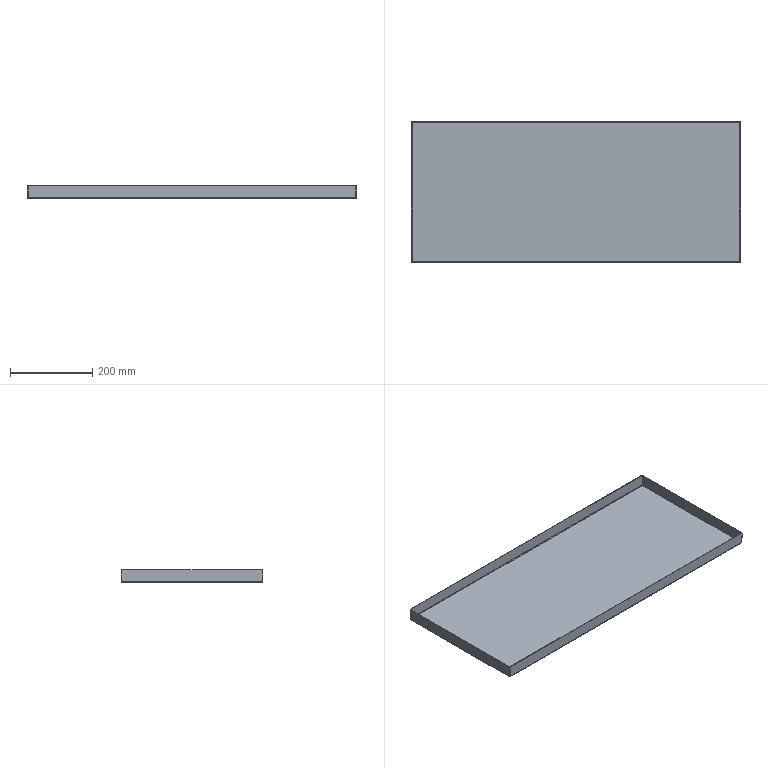Part | SolidWorks | features EdgeFlange 1, FlatPattern 1, SMBaseFlange 1, SheetMetal 1 | 1 solid | 38 faces | box 800 x 344 x 30 mm | volume 406893 mm3 | plane 22 | spline 8 | cylinder 8 | commonest cylinder face diameters 2 x4 4.4 x4
STEP:
#1=CARTESIAN_POINT('',(397.8,169.8,-1.2));
#2=VERTEX_POINT('',#1);
#3=CARTESIAN_POINT('',(397.8,-169.8,-1.2));
#4=VERTEX_POINT('',#3);
#5=CARTESIAN_POINT('',(397.8,170.093,-1.2));
#6=DIRECTION('',(0.,-1.,0.));
#7=VECTOR('',#6,1000.);
#8=LINE('',#5,#7);
#9=EDGE_CURVE('',#2,#4,#8,.T.);
#10=ORIENTED_EDGE('',*,*,#9,.T.);
#11=CARTESIAN_POINT('',(-397.8,-169.8,-1.2));
#12=VERTEX_POINT('',#11);
#13=CARTESIAN_POINT('',(398.093,-169.8,-1.2));
#14=DIRECTION('',(-1.,0.,0.));
#15=VECTOR('',#14,1000.);
#16=LINE('',#13,#15);
#17=EDGE_CURVE('',#4,#12,#16,.T.);
#18=ORIENTED_EDGE('',*,*,#17,.T.);
#19=CARTESIAN_POINT('',(-397.8,169.8,-1.2));
#20=VERTEX_POINT('',#19);
#21=CARTESIAN_POINT('',(-397.8,-170.093,-1.2));
#22=DIRECTION('',(0.,1.,0.));
#23=VECTOR('',#22,1000.);
#24=LINE('',#21,#23);
#25=EDGE_CURVE('',#12,#20,#24,.T.);
#26=ORIENTED_EDGE('',*,*,#25,.T.);
#27=CARTESIAN_POINT('',(-398.093,169.8,-1.2));
#28=DIRECTION('',(1.,0.,0.));
#29=VECTOR('',#28,1000.);
#30=LINE('',#27,#29);
#31=EDGE_CURVE('',#20,#2,#30,.T.);
#32=ORIENTED_EDGE('',*,*,#31,.T.);
#33=EDGE_LOOP('',(#10,#18,#26,#32));
#34=FACE_OUTER_BOUND('',#33,.T.);
#35=CARTESIAN_POINT('',(0.,0.,-1.2));
#36=DIRECTION('',(0.,0.,1.));
#37=DIRECTION('',(1.,0.,0.));
#38=AXIS2_PLACEMENT_3D('',#35,#36,#37);
#39=PLANE('',#38);
#40=ADVANCED_FACE('',(#34),#39,.F.);
#41=CARTESIAN_POINT('',(397.8,-169.8,0.));
#42=VERTEX_POINT('',#41);
#43=CARTESIAN_POINT('',(-397.8,-169.8,0.));
#44=VERTEX_POINT('',#43);
#45=CARTESIAN_POINT('',(398.093,-169.8,0.));
#46=DIRECTION('',(-1.,0.,0.));
#47=VECTOR('',#46,1000.);
#48=LINE('',#45,#47);
#49=EDGE_CURVE('',#42,#44,#48,.T.);
#50=ORIENTED_EDGE('',*,*,#49,.F.);
#51=CARTESIAN_POINT('',(397.8,169.8,0.));
#52=VERTEX_POINT('',#51);
#53=CARTESIAN_POINT('',(397.8,170.093,0.));
#54=DIRECTION('',(0.,-1.,0.));
#55=VECTOR('',#54,1000.);
#56=LINE('',#53,#55);
#57=EDGE_CURVE('',#52,#42,#56,.T.);
#58=ORIENTED_EDGE('',*,*,#57,.F.);
#59=CARTESIAN_POINT('',(-397.8,169.8,0.));
#60=VERTEX_POINT('',#59);
#61=CARTESIAN_POINT('',(-398.093,169.8,0.));
#62=DIRECTION('',(1.,0.,0.));
#63=VECTOR('',#62,1000.);
#64=LINE('',#61,#63);
#65=EDGE_CURVE('',#60,#52,#64,.T.);
#66=ORIENTED_EDGE('',*,*,#65,.F.);
#67=CARTESIAN_POINT('',(-397.8,-170.093,0.));
#68=DIRECTION('',(0.,1.,0.));
#69=VECTOR('',#68,1000.);
#70=LINE('',#67,#69);
#71=EDGE_CURVE('',#44,#60,#70,.T.);
#72=ORIENTED_EDGE('',*,*,#71,.F.);
#73=EDGE_LOOP('',(#50,#58,#66,#72));
#74=FACE_OUTER_BOUND('',#73,.T.);
#75=CARTESIAN_POINT('',(0.,0.,0.));
#76=DIRECTION('',(0.,0.,1.));
#77=DIRECTION('',(1.,0.,0.));
#78=AXIS2_PLACEMENT_3D('',#75,#76,#77);
#79=PLANE('',#78);
#80=ADVANCED_FACE('',(#74),#79,.T.);
#81=CARTESIAN_POINT('',(398.093,172.,1.));
#82=VERTEX_POINT('',#81);
#83=CARTESIAN_POINT('',(398.093,170.8,1.));
#84=VERTEX_POINT('',#83);
#85=CARTESIAN_POINT('',(398.093,170.8,1.));
#86=DIRECTION('',(0.,-1.,0.));
#87=VECTOR('',#86,1000.);
#88=LINE('',#85,#87);
#89=EDGE_CURVE('',#82,#84,#88,.T.);
#90=ORIENTED_EDGE('',*,*,#89,.T.);
#91=CARTESIAN_POINT('',(397.8,169.8,0.));
#92=CARTESIAN_POINT('',(397.849,170.062,0.));
#93=CARTESIAN_POINT('',(397.898,170.322,0.1078));
#94=CARTESIAN_POINT('',(397.995,170.692,0.478));
#95=CARTESIAN_POINT('',(398.044,170.8,0.7382));
#96=CARTESIAN_POINT('',(398.093,170.8,1.));
#97=B_SPLINE_CURVE_WITH_KNOTS('',3,(#91,#92,#93,#94,#95,#96),.UNSPECIFIED.,.F.,.F.,(4,2,4),(0.,0.5,1.),.UNSPECIFIED.);
#98=EDGE_CURVE('',#52,#84,#97,.T.);
#99=ORIENTED_EDGE('',*,*,#98,.F.);
#100=CARTESIAN_POINT('',(397.8,169.8,0.));
#101=DIRECTION('',(0.,0.,-1.));
#102=VECTOR('',#101,1000.);
#103=LINE('',#100,#102);
#104=EDGE_CURVE('',#52,#2,#103,.T.);
#105=ORIENTED_EDGE('',*,*,#104,.T.);
#106=CARTESIAN_POINT('',(397.8,169.8,-1.2));
#107=CARTESIAN_POINT('',(397.824,170.088,-1.2));
#108=CARTESIAN_POINT('',(397.849,170.376,-1.143));
#109=CARTESIAN_POINT('',(397.898,170.908,-0.9223));
#110=CARTESIAN_POINT('',(397.922,171.152,-0.7593));
#111=CARTESIAN_POINT('',(397.971,171.559,-0.352));
#112=CARTESIAN_POINT('',(397.995,171.722,-0.108));
#113=CARTESIAN_POINT('',(398.044,171.943,0.4242));
#114=CARTESIAN_POINT('',(398.068,172.,0.712));
#115=CARTESIAN_POINT('',(398.093,172.,1.));
#116=B_SPLINE_CURVE_WITH_KNOTS('',3,(#106,#107,#108,#109,#110,#111,#112,#113,#114,#115),.UNSPECIFIED.,.F.,.F.,(4,2,2,2,4),(0.,0.25,0.5,0.75,1.),.UNSPECIFIED.);
#117=EDGE_CURVE('',#2,#82,#116,.T.);
#118=ORIENTED_EDGE('',*,*,#117,.T.);
#119=EDGE_LOOP('',(#90,#99,#105,#118));
#120=FACE_OUTER_BOUND('',#119,.T.);
#121=CARTESIAN_POINT('',(397.8,169.8,-1.212));
#122=CARTESIAN_POINT('',(397.824,170.09,-1.212));
#123=CARTESIAN_POINT('',(397.849,170.379,-1.154));
#124=CARTESIAN_POINT('',(397.898,170.914,-0.9328));
#125=CARTESIAN_POINT('',(397.922,171.159,-0.7689));
#126=CARTESIAN_POINT('',(397.971,171.569,-0.3594));
#127=CARTESIAN_POINT('',(397.995,171.733,-0.114));
#128=CARTESIAN_POINT('',(398.044,171.954,0.421));
#129=CARTESIAN_POINT('',(398.068,172.012,0.7104));
#130=CARTESIAN_POINT('',(398.093,172.012,1.));
#131=CARTESIAN_POINT('',(397.8,169.8,-1.2));
#132=CARTESIAN_POINT('',(397.824,170.088,-1.2));
#133=CARTESIAN_POINT('',(397.849,170.376,-1.143));
#134=CARTESIAN_POINT('',(397.898,170.908,-0.9223));
#135=CARTESIAN_POINT('',(397.922,171.152,-0.7593));
#136=CARTESIAN_POINT('',(397.971,171.559,-0.352));
#137=CARTESIAN_POINT('',(397.995,171.722,-0.108));
#138=CARTESIAN_POINT('',(398.044,171.943,0.4242));
#139=CARTESIAN_POINT('',(398.068,172.,0.712));
#140=CARTESIAN_POINT('',(398.093,172.,1.));
#141=CARTESIAN_POINT('',(397.8,169.8,0.));
#142=CARTESIAN_POINT('',(397.824,169.931,0.));
#143=CARTESIAN_POINT('',(397.849,170.062,0.02603));
#144=CARTESIAN_POINT('',(397.898,170.304,0.1262));
#145=CARTESIAN_POINT('',(397.922,170.415,0.2003));
#146=CARTESIAN_POINT('',(397.971,170.6,0.3855));
#147=CARTESIAN_POINT('',(397.995,170.674,0.4964));
#148=CARTESIAN_POINT('',(398.044,170.774,0.7383));
#149=CARTESIAN_POINT('',(398.068,170.8,0.8691));
#150=CARTESIAN_POINT('',(398.093,170.8,1.));
#151=CARTESIAN_POINT('',(397.8,169.8,0.01212));
#152=CARTESIAN_POINT('',(397.824,169.929,0.01212));
#153=CARTESIAN_POINT('',(397.849,170.059,0.03783));
#154=CARTESIAN_POINT('',(397.898,170.298,0.1368));
#155=CARTESIAN_POINT('',(397.922,170.407,0.21));
#156=CARTESIAN_POINT('',(397.971,170.59,0.3929));
#157=CARTESIAN_POINT('',(397.995,170.663,0.5025));
#158=CARTESIAN_POINT('',(398.044,170.762,0.7414));
#159=CARTESIAN_POINT('',(398.068,170.788,0.8707));
#160=CARTESIAN_POINT('',(398.093,170.788,1.));
#161=B_SPLINE_SURFACE_WITH_KNOTS('',1,3,((#121,#122,#123,#124,#125,#126,#127,#128,#129,#130),(#131,#132,#133,#134,#135,#136,#137,#138,#139,#140),(#141,#142,#143,#144,#145,#146,#147,#148,#149,#150),(#151,#152,#153,#154,#155,#156,#157,#158,#159,#160)),.UNSPECIFIED.,.F.,.F.,.F.,(2,1,1,2),(4,2,2,2,4),(-0.01,0.,1.,1.01),(0.,0.25,0.5,0.75,1.),.UNSPECIFIED.);
#162=ADVANCED_FACE('',(#120),#161,.F.);
#163=CARTESIAN_POINT('',(-398.093,170.8,1.));
#164=VERTEX_POINT('',#163);
#165=CARTESIAN_POINT('',(-398.093,170.8,1.));
#166=CARTESIAN_POINT('',(-398.044,170.8,0.7382));
#167=CARTESIAN_POINT('',(-397.995,170.692,0.478));
#168=CARTESIAN_POINT('',(-397.898,170.322,0.1078));
#169=CARTESIAN_POINT('',(-397.849,170.062,0.));
#170=CARTESIAN_POINT('',(-397.8,169.8,0.));
#171=B_SPLINE_CURVE_WITH_KNOTS('',3,(#165,#166,#167,#168,#169,#170),.UNSPECIFIED.,.F.,.F.,(4,2,4),(0.,0.5,1.),.UNSPECIFIED.);
#172=EDGE_CURVE('',#164,#60,#171,.T.);
#173=ORIENTED_EDGE('',*,*,#172,.F.);
#174=CARTESIAN_POINT('',(-398.093,172.,1.));
#175=VERTEX_POINT('',#174);
#176=CARTESIAN_POINT('',(-398.093,170.8,1.));
#177=DIRECTION('',(0.,-1.,0.));
#178=VECTOR('',#177,1000.);
#179=LINE('',#176,#178);
#180=EDGE_CURVE('',#175,#164,#179,.T.);
#181=ORIENTED_EDGE('',*,*,#180,.F.);
#182=CARTESIAN_POINT('',(-398.093,172.,1.));
#183=CARTESIAN_POINT('',(-398.068,172.,0.712));
#184=CARTESIAN_POINT('',(-398.044,171.943,0.4242));
#185=CARTESIAN_POINT('',(-397.995,171.722,-0.108));
#186=CARTESIAN_POINT('',(-397.971,171.559,-0.352));
#187=CARTESIAN_POINT('',(-397.922,171.152,-0.7593));
#188=CARTESIAN_POINT('',(-397.898,170.908,-0.9223));
#189=CARTESIAN_POINT('',(-397.849,170.376,-1.143));
#190=CARTESIAN_POINT('',(-397.824,170.088,-1.2));
#191=CARTESIAN_POINT('',(-397.8,169.8,-1.2));
#192=B_SPLINE_CURVE_WITH_KNOTS('',3,(#182,#183,#184,#185,#186,#187,#188,#189,#190,#191),.UNSPECIFIED.,.F.,.F.,(4,2,2,2,4),(0.,0.25,0.5,0.75,1.),.UNSPECIFIED.);
#193=EDGE_CURVE('',#175,#20,#192,.T.);
#194=ORIENTED_EDGE('',*,*,#193,.T.);
#195=CARTESIAN_POINT('',(-397.8,169.8,0.));
#196=DIRECTION('',(0.,0.,-1.));
#197=VECTOR('',#196,1000.);
#198=LINE('',#195,#197);
#199=EDGE_CURVE('',#60,#20,#198,.T.);
#200=ORIENTED_EDGE('',*,*,#199,.F.);
#201=EDGE_LOOP('',(#173,#181,#194,#200));
#202=FACE_OUTER_BOUND('',#201,.T.);
#203=CARTESIAN_POINT('',(-398.093,172.012,1.));
#204=CARTESIAN_POINT('',(-398.068,172.012,0.7104));
#205=CARTESIAN_POINT('',(-398.044,171.954,0.421));
#206=CARTESIAN_POINT('',(-397.995,171.733,-0.114));
#207=CARTESIAN_POINT('',(-397.971,171.569,-0.3594));
#208=CARTESIAN_POINT('',(-397.922,171.159,-0.7689));
#209=CARTESIAN_POINT('',(-397.898,170.914,-0.9328));
#210=CARTESIAN_POINT('',(-397.849,170.379,-1.154));
#211=CARTESIAN_POINT('',(-397.824,170.09,-1.212));
#212=CARTESIAN_POINT('',(-397.8,169.8,-1.212));
#213=CARTESIAN_POINT('',(-398.093,172.,1.));
#214=CARTESIAN_POINT('',(-398.068,172.,0.712));
#215=CARTESIAN_POINT('',(-398.044,171.943,0.4242));
#216=CARTESIAN_POINT('',(-397.995,171.722,-0.108));
#217=CARTESIAN_POINT('',(-397.971,171.559,-0.352));
#218=CARTESIAN_POINT('',(-397.922,171.152,-0.7593));
#219=CARTESIAN_POINT('',(-397.898,170.908,-0.9223));
#220=CARTESIAN_POINT('',(-397.849,170.376,-1.143));
#221=CARTESIAN_POINT('',(-397.824,170.088,-1.2));
#222=CARTESIAN_POINT('',(-397.8,169.8,-1.2));
#223=CARTESIAN_POINT('',(-398.093,170.8,1.));
#224=CARTESIAN_POINT('',(-398.068,170.8,0.8691));
#225=CARTESIAN_POINT('',(-398.044,170.774,0.7383));
#226=CARTESIAN_POINT('',(-397.995,170.674,0.4964));
#227=CARTESIAN_POINT('',(-397.971,170.6,0.3855));
#228=CARTESIAN_POINT('',(-397.922,170.415,0.2003));
#229=CARTESIAN_POINT('',(-397.898,170.304,0.1262));
#230=CARTESIAN_POINT('',(-397.849,170.062,0.02603));
#231=CARTESIAN_POINT('',(-397.824,169.931,0.));
#232=CARTESIAN_POINT('',(-397.8,169.8,0.));
#233=CARTESIAN_POINT('',(-398.093,170.788,1.));
#234=CARTESIAN_POINT('',(-398.068,170.788,0.8707));
#235=CARTESIAN_POINT('',(-398.044,170.762,0.7414));
#236=CARTESIAN_POINT('',(-397.995,170.663,0.5025));
#237=CARTESIAN_POINT('',(-397.971,170.59,0.3929));
#238=CARTESIAN_POINT('',(-397.922,170.407,0.21));
#239=CARTESIAN_POINT('',(-397.898,170.298,0.1368));
#240=CARTESIAN_POINT('',(-397.849,170.059,0.03783));
#241=CARTESIAN_POINT('',(-397.824,169.929,0.01212));
#242=CARTESIAN_POINT('',(-397.8,169.8,0.01212));
#243=B_SPLINE_SURFACE_WITH_KNOTS('',1,3,((#203,#204,#205,#206,#207,#208,#209,#210,#211,#212),(#213,#214,#215,#216,#217,#218,#219,#220,#221,#222),(#223,#224,#225,#226,#227,#228,#229,#230,#231,#232),(#233,#234,#235,#236,#237,#238,#239,#240,#241,#242)),.UNSPECIFIED.,.F.,.F.,.F.,(2,1,1,2),(4,2,2,2,4),(-0.01,0.,1.,1.01),(0.,0.25,0.5,0.75,1.),.UNSPECIFIED.);
#244=ADVANCED_FACE('',(#202),#243,.F.);
#245=ORIENTED_EDGE('',*,*,#31,.F.);
#246=ORIENTED_EDGE('',*,*,#193,.F.);
#247=CARTESIAN_POINT('',(400.,172.,1.));
#248=DIRECTION('',(1.,0.,0.));
#249=VECTOR('',#248,1000.);
#250=LINE('',#247,#249);
#251=EDGE_CURVE('',#175,#82,#250,.T.);
#252=ORIENTED_EDGE('',*,*,#251,.T.);
#253=ORIENTED_EDGE('',*,*,#117,.F.);
#254=EDGE_LOOP('',(#245,#246,#252,#253));
#255=FACE_OUTER_BOUND('',#254,.T.);
#256=CARTESIAN_POINT('',(-398.093,169.8,1.));
#257=DIRECTION('',(-1.,0.,0.));
#258=DIRECTION('',(0.,1.,0.));
#259=AXIS2_PLACEMENT_3D('',#256,#257,#258);
#260=CYLINDRICAL_SURFACE('',#259,2.2);
#261=ADVANCED_FACE('',(#255),#260,.T.);
#262=ORIENTED_EDGE('',*,*,#65,.T.);
#263=ORIENTED_EDGE('',*,*,#98,.T.);
#264=CARTESIAN_POINT('',(400.,170.8,1.));
#265=DIRECTION('',(-1.,0.,0.));
#266=VECTOR('',#265,1000.);
#267=LINE('',#264,#266);
#268=EDGE_CURVE('',#84,#164,#267,.T.);
#269=ORIENTED_EDGE('',*,*,#268,.T.);
#270=ORIENTED_EDGE('',*,*,#172,.T.);
#271=EDGE_LOOP('',(#262,#263,#269,#270));
#272=FACE_OUTER_BOUND('',#271,.T.);
#273=CARTESIAN_POINT('',(-398.093,169.8,1.));
#274=DIRECTION('',(-1.,0.,0.));
#275=DIRECTION('',(0.,1.,0.));
#276=AXIS2_PLACEMENT_3D('',#273,#274,#275);
#277=CYLINDRICAL_SURFACE('',#276,1.);
#278=ADVANCED_FACE('',(#272),#277,.F.);
#279=CARTESIAN_POINT('',(398.093,172.,28.8));
#280=VERTEX_POINT('',#279);
#281=CARTESIAN_POINT('',(398.093,172.,0.));
#282=DIRECTION('',(0.,0.,1.));
#283=VECTOR('',#282,1000.);
#284=LINE('',#281,#283);
#285=EDGE_CURVE('',#82,#280,#284,.T.);
#286=ORIENTED_EDGE('',*,*,#285,.T.);
#287=CARTESIAN_POINT('',(398.093,170.8,28.8));
#288=VERTEX_POINT('',#287);
#289=CARTESIAN_POINT('',(398.093,170.8,28.8));
#290=DIRECTION('',(0.,-1.,0.));
#291=VECTOR('',#290,1000.);
#292=LINE('',#289,#291);
#293=EDGE_CURVE('',#280,#288,#292,.T.);
#294=ORIENTED_EDGE('',*,*,#293,.T.);
#295=CARTESIAN_POINT('',(398.093,170.8,0.));
#296=DIRECTION('',(0.,0.,1.));
#297=VECTOR('',#296,1000.);
#298=LINE('',#295,#297);
#299=EDGE_CURVE('',#84,#288,#298,.T.);
#300=ORIENTED_EDGE('',*,*,#299,.F.);
#301=ORIENTED_EDGE('',*,*,#89,.F.);
#302=EDGE_LOOP('',(#286,#294,#300,#301));
#303=FACE_OUTER_BOUND('',#302,.T.);
#304=CARTESIAN_POINT('',(398.093,170.8,0.));
#305=DIRECTION('',(1.,0.,0.));
#306=DIRECTION('',(0.,0.,-1.));
#307=AXIS2_PLACEMENT_3D('',#304,#305,#306);
#308=PLANE('',#307);
#309=ADVANCED_FACE('',(#303),#308,.T.);
#310=ORIENTED_EDGE('',*,*,#251,.F.);
#311=CARTESIAN_POINT('',(-398.093,172.,28.8));
#312=VERTEX_POINT('',#311);
#313=CARTESIAN_POINT('',(-398.093,172.,0.));
#314=DIRECTION('',(0.,0.,1.));
#315=VECTOR('',#314,1000.);
#316=LINE('',#313,#315);
#317=EDGE_CURVE('',#175,#312,#316,.T.);
#318=ORIENTED_EDGE('',*,*,#317,.T.);
#319=CARTESIAN_POINT('',(0.,172.,28.8));
#320=DIRECTION('',(1.,0.,0.));
#321=VECTOR('',#320,1000.);
#322=LINE('',#319,#321);
#323=EDGE_CURVE('',#312,#280,#322,.T.);
#324=ORIENTED_EDGE('',*,*,#323,.T.);
#325=ORIENTED_EDGE('',*,*,#285,.F.);
#326=EDGE_LOOP('',(#310,#318,#324,#325));
#327=FACE_OUTER_BOUND('',#326,.T.);
#328=CARTESIAN_POINT('',(0.,172.,0.));
#329=DIRECTION('',(0.,-1.,0.));
#330=DIRECTION('',(0.,0.,-1.));
#331=AXIS2_PLACEMENT_3D('',#328,#329,#330);
#332=PLANE('',#331);
#333=ADVANCED_FACE('',(#327),#332,.F.);
#334=CARTESIAN_POINT('',(-398.093,170.8,28.8));
#335=VERTEX_POINT('',#334);
#336=CARTESIAN_POINT('',(-398.093,170.8,0.));
#337=DIRECTION('',(0.,0.,1.));
#338=VECTOR('',#337,1000.);
#339=LINE('',#336,#338);
#340=EDGE_CURVE('',#164,#335,#339,.T.);
#341=ORIENTED_EDGE('',*,*,#340,.F.);
#342=ORIENTED_EDGE('',*,*,#268,.F.);
#343=ORIENTED_EDGE('',*,*,#299,.T.);
#344=CARTESIAN_POINT('',(400.,170.8,28.8));
#345=DIRECTION('',(1.,0.,0.));
#346=VECTOR('',#345,1000.);
#347=LINE('',#344,#346);
#348=EDGE_CURVE('',#335,#288,#347,.T.);
#349=ORIENTED_EDGE('',*,*,#348,.F.);
#350=EDGE_LOOP('',(#341,#342,#343,#349));
#351=FACE_OUTER_BOUND('',#350,.T.);
#352=CARTESIAN_POINT('',(0.,170.8,0.));
#353=DIRECTION('',(0.,-1.,0.));
#354=DIRECTION('',(0.,0.,-1.));
#355=AXIS2_PLACEMENT_3D('',#352,#353,#354);
#356=PLANE('',#355);
#357=ADVANCED_FACE('',(#351),#356,.T.);
#358=ORIENTED_EDGE('',*,*,#323,.F.);
#359=CARTESIAN_POINT('',(-398.093,172.,28.8));
#360=DIRECTION('',(0.,-1.,0.));
#361=VECTOR('',#360,1000.);
#362=LINE('',#359,#361);
#363=EDGE_CURVE('',#312,#335,#362,.T.);
#364=ORIENTED_EDGE('',*,*,#363,.T.);
#365=ORIENTED_EDGE('',*,*,#348,.T.);
#366=ORIENTED_EDGE('',*,*,#293,.F.);
#367=EDGE_LOOP('',(#358,#364,#365,#366));
#368=FACE_OUTER_BOUND('',#367,.T.);
#369=CARTESIAN_POINT('',(400.,172.,28.8));
#370=DIRECTION('',(0.,0.,-1.));
#371=DIRECTION('',(0.,1.,0.));
#372=AXIS2_PLACEMENT_3D('',#369,#370,#371);
#373=PLANE('',#372);
#374=ADVANCED_FACE('',(#368),#373,.F.);
#375=ORIENTED_EDGE('',*,*,#363,.F.);
#376=ORIENTED_EDGE('',*,*,#317,.F.);
#377=ORIENTED_EDGE('',*,*,#180,.T.);
#378=ORIENTED_EDGE('',*,*,#340,.T.);
#379=EDGE_LOOP('',(#375,#376,#377,#378));
#380=FACE_OUTER_BOUND('',#379,.T.);
#381=CARTESIAN_POINT('',(-398.093,170.8,0.));
#382=DIRECTION('',(1.,0.,0.));
#383=DIRECTION('',(0.,0.,-1.));
#384=AXIS2_PLACEMENT_3D('',#381,#382,#383);
#385=PLANE('',#384);
#386=ADVANCED_FACE('',(#380),#385,.F.);
#387=CARTESIAN_POINT('',(-400.,170.093,1.));
#388=VERTEX_POINT('',#387);
#389=CARTESIAN_POINT('',(-398.8,170.093,1.));
#390=VERTEX_POINT('',#389);
#391=CARTESIAN_POINT('',(-398.8,170.093,1.));
#392=DIRECTION('',(1.,0.,0.));
#393=VECTOR('',#392,1000.);
#394=LINE('',#391,#393);
#395=EDGE_CURVE('',#388,#390,#394,.T.);
#396=ORIENTED_EDGE('',*,*,#395,.T.);
#397=CARTESIAN_POINT('',(-397.8,169.8,0.));
#398=CARTESIAN_POINT('',(-398.062,169.849,0.));
#399=CARTESIAN_POINT('',(-398.322,169.898,0.1078));
#400=CARTESIAN_POINT('',(-398.692,169.995,0.478));
#401=CARTESIAN_POINT('',(-398.8,170.044,0.7382));
#402=CARTESIAN_POINT('',(-398.8,170.093,1.));
#403=B_SPLINE_CURVE_WITH_KNOTS('',3,(#397,#398,#399,#400,#401,#402),.UNSPECIFIED.,.F.,.F.,(4,2,4),(0.,0.5,1.),.UNSPECIFIED.);
#404=EDGE_CURVE('',#60,#390,#403,.T.);
#405=ORIENTED_EDGE('',*,*,#404,.F.);
#406=ORIENTED_EDGE('',*,*,#199,.T.);
#407=CARTESIAN_POINT('',(-397.8,169.8,-1.2));
#408=CARTESIAN_POINT('',(-398.088,169.824,-1.2));
#409=CARTESIAN_POINT('',(-398.376,169.849,-1.143));
#410=CARTESIAN_POINT('',(-398.908,169.898,-0.9223));
#411=CARTESIAN_POINT('',(-399.152,169.922,-0.7593));
#412=CARTESIAN_POINT('',(-399.559,169.971,-0.352));
#413=CARTESIAN_POINT('',(-399.722,169.995,-0.108));
#414=CARTESIAN_POINT('',(-399.943,170.044,0.4242));
#415=CARTESIAN_POINT('',(-400.,170.068,0.712));
#416=CARTESIAN_POINT('',(-400.,170.093,1.));
#417=B_SPLINE_CURVE_WITH_KNOTS('',3,(#407,#408,#409,#410,#411,#412,#413,#414,#415,#416),.UNSPECIFIED.,.F.,.F.,(4,2,2,2,4),(0.,0.25,0.5,0.75,1.),.UNSPECIFIED.);
#418=EDGE_CURVE('',#20,#388,#417,.T.);
#419=ORIENTED_EDGE('',*,*,#418,.T.);
#420=EDGE_LOOP('',(#396,#405,#406,#419));
#421=FACE_OUTER_BOUND('',#420,.T.);
#422=CARTESIAN_POINT('',(-397.8,169.8,-1.212));
#423=CARTESIAN_POINT('',(-398.09,169.824,-1.212));
#424=CARTESIAN_POINT('',(-398.379,169.849,-1.154));
#425=CARTESIAN_POINT('',(-398.914,169.898,-0.9328));
#426=CARTESIAN_POINT('',(-399.159,169.922,-0.7689));
#427=CARTESIAN_POINT('',(-399.569,169.971,-0.3594));
#428=CARTESIAN_POINT('',(-399.733,169.995,-0.114));
#429=CARTESIAN_POINT('',(-399.954,170.044,0.421));
#430=CARTESIAN_POINT('',(-400.012,170.068,0.7104));
#431=CARTESIAN_POINT('',(-400.012,170.093,1.));
#432=CARTESIAN_POINT('',(-397.8,169.8,-1.2));
#433=CARTESIAN_POINT('',(-398.088,169.824,-1.2));
#434=CARTESIAN_POINT('',(-398.376,169.849,-1.143));
#435=CARTESIAN_POINT('',(-398.908,169.898,-0.9223));
#436=CARTESIAN_POINT('',(-399.152,169.922,-0.7593));
#437=CARTESIAN_POINT('',(-399.559,169.971,-0.352));
#438=CARTESIAN_POINT('',(-399.722,169.995,-0.108));
#439=CARTESIAN_POINT('',(-399.943,170.044,0.4242));
#440=CARTESIAN_POINT('',(-400.,170.068,0.712));
#441=CARTESIAN_POINT('',(-400.,170.093,1.));
#442=CARTESIAN_POINT('',(-397.8,169.8,0.));
#443=CARTESIAN_POINT('',(-397.931,169.824,0.));
#444=CARTESIAN_POINT('',(-398.062,169.849,0.02603));
#445=CARTESIAN_POINT('',(-398.304,169.898,0.1262));
#446=CARTESIAN_POINT('',(-398.415,169.922,0.2003));
#447=CARTESIAN_POINT('',(-398.6,169.971,0.3855));
#448=CARTESIAN_POINT('',(-398.674,169.995,0.4964));
#449=CARTESIAN_POINT('',(-398.774,170.044,0.7383));
#450=CARTESIAN_POINT('',(-398.8,170.068,0.8691));
#451=CARTESIAN_POINT('',(-398.8,170.093,1.));
#452=CARTESIAN_POINT('',(-397.8,169.8,0.01212));
#453=CARTESIAN_POINT('',(-397.929,169.824,0.01212));
#454=CARTESIAN_POINT('',(-398.059,169.849,0.03783));
#455=CARTESIAN_POINT('',(-398.298,169.898,0.1368));
#456=CARTESIAN_POINT('',(-398.407,169.922,0.21));
#457=CARTESIAN_POINT('',(-398.59,169.971,0.3929));
#458=CARTESIAN_POINT('',(-398.663,169.995,0.5025));
#459=CARTESIAN_POINT('',(-398.762,170.044,0.7414));
#460=CARTESIAN_POINT('',(-398.788,170.068,0.8707));
#461=CARTESIAN_POINT('',(-398.788,170.093,1.));
#462=B_SPLINE_SURFACE_WITH_KNOTS('',1,3,((#422,#423,#424,#425,#426,#427,#428,#429,#430,#431),(#432,#433,#434,#435,#436,#437,#438,#439,#440,#441),(#442,#443,#444,#445,#446,#447,#448,#449,#450,#451),(#452,#453,#454,#455,#456,#457,#458,#459,#460,#461)),.UNSPECIFIED.,.F.,.F.,.F.,(2,1,1,2),(4,2,2,2,4),(-0.01,0.,1.,1.01),(0.,0.25,0.5,0.75,1.),.UNSPECIFIED.);
#463=ADVANCED_FACE('',(#421),#462,.F.);
#464=CARTESIAN_POINT('',(-398.8,-170.093,1.));
#465=VERTEX_POINT('',#464);
#466=CARTESIAN_POINT('',(-398.8,-170.093,1.));
#467=CARTESIAN_POINT('',(-398.8,-170.044,0.7382));
#468=CARTESIAN_POINT('',(-398.692,-169.995,0.478));
#469=CARTESIAN_POINT('',(-398.322,-169.898,0.1078));
#470=CARTESIAN_POINT('',(-398.062,-169.849,0.));
#471=CARTESIAN_POINT('',(-397.8,-169.8,0.));
#472=B_SPLINE_CURVE_WITH_KNOTS('',3,(#466,#467,#468,#469,#470,#471),.UNSPECIFIED.,.F.,.F.,(4,2,4),(0.,0.5,1.),.UNSPECIFIED.);
#473=EDGE_CURVE('',#465,#44,#472,.T.);
#474=ORIENTED_EDGE('',*,*,#473,.F.);
#475=CARTESIAN_POINT('',(-400.,-170.093,1.));
#476=VERTEX_POINT('',#475);
#477=CARTESIAN_POINT('',(-398.8,-170.093,1.));
#478=DIRECTION('',(1.,0.,0.));
#479=VECTOR('',#478,1000.);
#480=LINE('',#477,#479);
#481=EDGE_CURVE('',#476,#465,#480,.T.);
#482=ORIENTED_EDGE('',*,*,#481,.F.);
#483=CARTESIAN_POINT('',(-400.,-170.093,1.));
#484=CARTESIAN_POINT('',(-400.,-170.068,0.712));
#485=CARTESIAN_POINT('',(-399.943,-170.044,0.4242));
#486=CARTESIAN_POINT('',(-399.722,-169.995,-0.108));
#487=CARTESIAN_POINT('',(-399.559,-169.971,-0.352));
#488=CARTESIAN_POINT('',(-399.152,-169.922,-0.7593));
#489=CARTESIAN_POINT('',(-398.908,-169.898,-0.9223));
#490=CARTESIAN_POINT('',(-398.376,-169.849,-1.143));
#491=CARTESIAN_POINT('',(-398.088,-169.824,-1.2));
#492=CARTESIAN_POINT('',(-397.8,-169.8,-1.2));
#493=B_SPLINE_CURVE_WITH_KNOTS('',3,(#483,#484,#485,#486,#487,#488,#489,#490,#491,#492),.UNSPECIFIED.,.F.,.F.,(4,2,2,2,4),(0.,0.25,0.5,0.75,1.),.UNSPECIFIED.);
#494=EDGE_CURVE('',#476,#12,#493,.T.);
#495=ORIENTED_EDGE('',*,*,#494,.T.);
#496=CARTESIAN_POINT('',(-397.8,-169.8,0.));
#497=DIRECTION('',(0.,0.,-1.));
#498=VECTOR('',#497,1000.);
#499=LINE('',#496,#498);
#500=EDGE_CURVE('',#44,#12,#499,.T.);
#501=ORIENTED_EDGE('',*,*,#500,.F.);
#502=EDGE_LOOP('',(#474,#482,#495,#501));
#503=FACE_OUTER_BOUND('',#502,.T.);
#504=CARTESIAN_POINT('',(-400.012,-170.093,1.));
#505=CARTESIAN_POINT('',(-400.012,-170.068,0.7104));
#506=CARTESIAN_POINT('',(-399.954,-170.044,0.421));
#507=CARTESIAN_POINT('',(-399.733,-169.995,-0.114));
#508=CARTESIAN_POINT('',(-399.569,-169.971,-0.3594));
#509=CARTESIAN_POINT('',(-399.159,-169.922,-0.7689));
#510=CARTESIAN_POINT('',(-398.914,-169.898,-0.9328));
#511=CARTESIAN_POINT('',(-398.379,-169.849,-1.154));
#512=CARTESIAN_POINT('',(-398.09,-169.824,-1.212));
#513=CARTESIAN_POINT('',(-397.8,-169.8,-1.212));
#514=CARTESIAN_POINT('',(-400.,-170.093,1.));
#515=CARTESIAN_POINT('',(-400.,-170.068,0.712));
#516=CARTESIAN_POINT('',(-399.943,-170.044,0.4242));
#517=CARTESIAN_POINT('',(-399.722,-169.995,-0.108));
#518=CARTESIAN_POINT('',(-399.559,-169.971,-0.352));
#519=CARTESIAN_POINT('',(-399.152,-169.922,-0.7593));
#520=CARTESIAN_POINT('',(-398.908,-169.898,-0.9223));
#521=CARTESIAN_POINT('',(-398.376,-169.849,-1.143));
#522=CARTESIAN_POINT('',(-398.088,-169.824,-1.2));
#523=CARTESIAN_POINT('',(-397.8,-169.8,-1.2));
#524=CARTESIAN_POINT('',(-398.8,-170.093,1.));
#525=CARTESIAN_POINT('',(-398.8,-170.068,0.8691));
#526=CARTESIAN_POINT('',(-398.774,-170.044,0.7383));
#527=CARTESIAN_POINT('',(-398.674,-169.995,0.4964));
#528=CARTESIAN_POINT('',(-398.6,-169.971,0.3855));
#529=CARTESIAN_POINT('',(-398.415,-169.922,0.2003));
#530=CARTESIAN_POINT('',(-398.304,-169.898,0.1262));
#531=CARTESIAN_POINT('',(-398.062,-169.849,0.02603));
#532=CARTESIAN_POINT('',(-397.931,-169.824,0.));
#533=CARTESIAN_POINT('',(-397.8,-169.8,0.));
#534=CARTESIAN_POINT('',(-398.788,-170.093,1.));
#535=CARTESIAN_POINT('',(-398.788,-170.068,0.8707));
#536=CARTESIAN_POINT('',(-398.762,-170.044,0.7414));
#537=CARTESIAN_POINT('',(-398.663,-169.995,0.5025));
#538=CARTESIAN_POINT('',(-398.59,-169.971,0.3929));
#539=CARTESIAN_POINT('',(-398.407,-169.922,0.21));
#540=CARTESIAN_POINT('',(-398.298,-169.898,0.1368));
#541=CARTESIAN_POINT('',(-398.059,-169.849,0.03783));
#542=CARTESIAN_POINT('',(-397.929,-169.824,0.01212));
#543=CARTESIAN_POINT('',(-397.8,-169.8,0.01212));
#544=B_SPLINE_SURFACE_WITH_KNOTS('',1,3,((#504,#505,#506,#507,#508,#509,#510,#511,#512,#513),(#514,#515,#516,#517,#518,#519,#520,#521,#522,#523),(#524,#525,#526,#527,#528,#529,#530,#531,#532,#533),(#534,#535,#536,#537,#538,#539,#540,#541,#542,#543)),.UNSPECIFIED.,.F.,.F.,.F.,(2,1,1,2),(4,2,2,2,4),(-0.01,0.,1.,1.01),(0.,0.25,0.5,0.75,1.),.UNSPECIFIED.);
#545=ADVANCED_FACE('',(#503),#544,.F.);
#546=ORIENTED_EDGE('',*,*,#25,.F.);
#547=ORIENTED_EDGE('',*,*,#494,.F.);
#548=CARTESIAN_POINT('',(-400.,172.,1.));
#549=DIRECTION('',(0.,1.,0.));
#550=VECTOR('',#549,1000.);
#551=LINE('',#548,#550);
#552=EDGE_CURVE('',#476,#388,#551,.T.);
#553=ORIENTED_EDGE('',*,*,#552,.T.);
#554=ORIENTED_EDGE('',*,*,#418,.F.);
#555=EDGE_LOOP('',(#546,#547,#553,#554));
#556=FACE_OUTER_BOUND('',#555,.T.);
#557=CARTESIAN_POINT('',(-397.8,-170.093,1.));
#558=DIRECTION('',(0.,-1.,0.));
#559=DIRECTION('',(-1.,0.,0.));
#560=AXIS2_PLACEMENT_3D('',#557,#558,#559);
#561=CYLINDRICAL_SURFACE('',#560,2.2);
#562=ADVANCED_FACE('',(#556),#561,.T.);
#563=ORIENTED_EDGE('',*,*,#71,.T.);
#564=ORIENTED_EDGE('',*,*,#404,.T.);
#565=CARTESIAN_POINT('',(-398.8,172.,1.));
#566=DIRECTION('',(0.,-1.,0.));
#567=VECTOR('',#566,1000.);
#568=LINE('',#565,#567);
#569=EDGE_CURVE('',#390,#465,#568,.T.);
#570=ORIENTED_EDGE('',*,*,#569,.T.);
#571=ORIENTED_EDGE('',*,*,#473,.T.);
#572=EDGE_LOOP('',(#563,#564,#570,#571));
#573=FACE_OUTER_BOUND('',#572,.T.);
#574=CARTESIAN_POINT('',(-397.8,-170.093,1.));
#575=DIRECTION('',(0.,-1.,0.));
#576=DIRECTION('',(-1.,0.,0.));
#577=AXIS2_PLACEMENT_3D('',#574,#575,#576);
#578=CYLINDRICAL_SURFACE('',#577,1.);
#579=ADVANCED_FACE('',(#573),#578,.F.);
#580=CARTESIAN_POINT('',(-400.,170.093,28.8));
#581=VERTEX_POINT('',#580);
#582=CARTESIAN_POINT('',(-400.,170.093,0.));
#583=DIRECTION('',(0.,0.,1.));
#584=VECTOR('',#583,1000.);
#585=LINE('',#582,#584);
#586=EDGE_CURVE('',#388,#581,#585,.T.);
#587=ORIENTED_EDGE('',*,*,#586,.T.);
#588=CARTESIAN_POINT('',(-398.8,170.093,28.8));
#589=VERTEX_POINT('',#588);
#590=CARTESIAN_POINT('',(-398.8,170.093,28.8));
#591=DIRECTION('',(1.,0.,0.));
#592=VECTOR('',#591,1000.);
#593=LINE('',#590,#592);
#594=EDGE_CURVE('',#581,#589,#593,.T.);
#595=ORIENTED_EDGE('',*,*,#594,.T.);
#596=CARTESIAN_POINT('',(-398.8,170.093,0.));
#597=DIRECTION('',(0.,0.,1.));
#598=VECTOR('',#597,1000.);
#599=LINE('',#596,#598);
#600=EDGE_CURVE('',#390,#589,#599,.T.);
#601=ORIENTED_EDGE('',*,*,#600,.F.);
#602=ORIENTED_EDGE('',*,*,#395,.F.);
#603=EDGE_LOOP('',(#587,#595,#601,#602));
#604=FACE_OUTER_BOUND('',#603,.T.);
#605=CARTESIAN_POINT('',(-398.8,170.093,0.));
#606=DIRECTION('',(0.,1.,0.));
#607=DIRECTION('',(0.,0.,1.));
#608=AXIS2_PLACEMENT_3D('',#605,#606,#607);
#609=PLANE('',#608);
#610=ADVANCED_FACE('',(#604),#609,.T.);
#611=ORIENTED_EDGE('',*,*,#552,.F.);
#612=CARTESIAN_POINT('',(-400.,-170.093,28.8));
#613=VERTEX_POINT('',#612);
#614=CARTESIAN_POINT('',(-400.,-170.093,0.));
#615=DIRECTION('',(0.,0.,1.));
#616=VECTOR('',#615,1000.);
#617=LINE('',#614,#616);
#618=EDGE_CURVE('',#476,#613,#617,.T.);
#619=ORIENTED_EDGE('',*,*,#618,.T.);
#620=CARTESIAN_POINT('',(-400.,0.,28.8));
#621=DIRECTION('',(0.,1.,0.));
#622=VECTOR('',#621,1000.);
#623=LINE('',#620,#622);
#624=EDGE_CURVE('',#613,#581,#623,.T.);
#625=ORIENTED_EDGE('',*,*,#624,.T.);
#626=ORIENTED_EDGE('',*,*,#586,.F.);
#627=EDGE_LOOP('',(#611,#619,#625,#626));
#628=FACE_OUTER_BOUND('',#627,.T.);
#629=CARTESIAN_POINT('',(-400.,0.,0.));
#630=DIRECTION('',(1.,0.,0.));
#631=DIRECTION('',(0.,0.,-1.));
#632=AXIS2_PLACEMENT_3D('',#629,#630,#631);
#633=PLANE('',#632);
#634=ADVANCED_FACE('',(#628),#633,.F.);
#635=CARTESIAN_POINT('',(-398.8,-170.093,28.8));
#636=VERTEX_POINT('',#635);
#637=CARTESIAN_POINT('',(-398.8,-170.093,0.));
#638=DIRECTION('',(0.,0.,1.));
#639=VECTOR('',#638,1000.);
#640=LINE('',#637,#639);
#641=EDGE_CURVE('',#465,#636,#640,.T.);
#642=ORIENTED_EDGE('',*,*,#641,.F.);
#643=ORIENTED_EDGE('',*,*,#569,.F.);
#644=ORIENTED_EDGE('',*,*,#600,.T.);
#645=CARTESIAN_POINT('',(-398.8,172.,28.8));
#646=DIRECTION('',(0.,1.,0.));
#647=VECTOR('',#646,1000.);
#648=LINE('',#645,#647);
#649=EDGE_CURVE('',#636,#589,#648,.T.);
#650=ORIENTED_EDGE('',*,*,#649,.F.);
#651=EDGE_LOOP('',(#642,#643,#644,#650));
#652=FACE_OUTER_BOUND('',#651,.T.);
#653=CARTESIAN_POINT('',(-398.8,0.,0.));
#654=DIRECTION('',(1.,0.,0.));
#655=DIRECTION('',(0.,0.,-1.));
#656=AXIS2_PLACEMENT_3D('',#653,#654,#655);
#657=PLANE('',#656);
#658=ADVANCED_FACE('',(#652),#657,.T.);
#659=ORIENTED_EDGE('',*,*,#624,.F.);
#660=CARTESIAN_POINT('',(-400.,-170.093,28.8));
#661=DIRECTION('',(1.,0.,0.));
#662=VECTOR('',#661,1000.);
#663=LINE('',#660,#662);
#664=EDGE_CURVE('',#613,#636,#663,.T.);
#665=ORIENTED_EDGE('',*,*,#664,.T.);
#666=ORIENTED_EDGE('',*,*,#649,.T.);
#667=ORIENTED_EDGE('',*,*,#594,.F.);
#668=EDGE_LOOP('',(#659,#665,#666,#667));
#669=FACE_OUTER_BOUND('',#668,.T.);
#670=CARTESIAN_POINT('',(-400.,172.,28.8));
#671=DIRECTION('',(0.,0.,-1.));
#672=DIRECTION('',(-1.,0.,0.));
#673=AXIS2_PLACEMENT_3D('',#670,#671,#672);
#674=PLANE('',#673);
#675=ADVANCED_FACE('',(#669),#674,.F.);
#676=ORIENTED_EDGE('',*,*,#664,.F.);
#677=ORIENTED_EDGE('',*,*,#618,.F.);
#678=ORIENTED_EDGE('',*,*,#481,.T.);
#679=ORIENTED_EDGE('',*,*,#641,.T.);
#680=EDGE_LOOP('',(#676,#677,#678,#679));
#681=FACE_OUTER_BOUND('',#680,.T.);
#682=CARTESIAN_POINT('',(-398.8,-170.093,0.));
#683=DIRECTION('',(0.,1.,0.));
#684=DIRECTION('',(0.,0.,1.));
#685=AXIS2_PLACEMENT_3D('',#682,#683,#684);
#686=PLANE('',#685);
#687=ADVANCED_FACE('',(#681),#686,.F.);
#688=CARTESIAN_POINT('',(-398.093,-172.,1.));
#689=VERTEX_POINT('',#688);
#690=CARTESIAN_POINT('',(-398.093,-170.8,1.));
#691=VERTEX_POINT('',#690);
#692=CARTESIAN_POINT('',(-398.093,-170.8,1.));
#693=DIRECTION('',(0.,1.,0.));
#694=VECTOR('',#693,1000.);
#695=LINE('',#692,#694);
#696=EDGE_CURVE('',#689,#691,#695,.T.);
#697=ORIENTED_EDGE('',*,*,#696,.T.);
#698=CARTESIAN_POINT('',(-397.8,-169.8,0.));
#699=CARTESIAN_POINT('',(-397.849,-170.062,0.));
#700=CARTESIAN_POINT('',(-397.898,-170.322,0.1078));
#701=CARTESIAN_POINT('',(-397.995,-170.692,0.478));
#702=CARTESIAN_POINT('',(-398.044,-170.8,0.7382));
#703=CARTESIAN_POINT('',(-398.093,-170.8,1.));
#704=B_SPLINE_CURVE_WITH_KNOTS('',3,(#698,#699,#700,#701,#702,#703),.UNSPECIFIED.,.F.,.F.,(4,2,4),(0.,0.5,1.),.UNSPECIFIED.);
#705=EDGE_CURVE('',#44,#691,#704,.T.);
#706=ORIENTED_EDGE('',*,*,#705,.F.);
#707=ORIENTED_EDGE('',*,*,#500,.T.);
#708=CARTESIAN_POINT('',(-397.8,-169.8,-1.2));
#709=CARTESIAN_POINT('',(-397.824,-170.088,-1.2));
#710=CARTESIAN_POINT('',(-397.849,-170.376,-1.143));
#711=CARTESIAN_POINT('',(-397.898,-170.908,-0.9223));
#712=CARTESIAN_POINT('',(-397.922,-171.152,-0.7593));
#713=CARTESIAN_POINT('',(-397.971,-171.559,-0.352));
#714=CARTESIAN_POINT('',(-397.995,-171.722,-0.108));
#715=CARTESIAN_POINT('',(-398.044,-171.943,0.4242));
#716=CARTESIAN_POINT('',(-398.068,-172.,0.712));
#717=CARTESIAN_POINT('',(-398.093,-172.,1.));
#718=B_SPLINE_CURVE_WITH_KNOTS('',3,(#708,#709,#710,#711,#712,#713,#714,#715,#716,#717),.UNSPECIFIED.,.F.,.F.,(4,2,2,2,4),(0.,0.25,0.5,0.75,1.),.UNSPECIFIED.);
#719=EDGE_CURVE('',#12,#689,#718,.T.);
#720=ORIENTED_EDGE('',*,*,#719,.T.);
#721=EDGE_LOOP('',(#697,#706,#707,#720));
#722=FACE_OUTER_BOUND('',#721,.T.);
#723=CARTESIAN_POINT('',(-397.8,-169.8,-1.212));
#724=CARTESIAN_POINT('',(-397.824,-170.09,-1.212));
#725=CARTESIAN_POINT('',(-397.849,-170.379,-1.154));
#726=CARTESIAN_POINT('',(-397.898,-170.914,-0.9328));
#727=CARTESIAN_POINT('',(-397.922,-171.159,-0.7689));
#728=CARTESIAN_POINT('',(-397.971,-171.569,-0.3594));
#729=CARTESIAN_POINT('',(-397.995,-171.733,-0.114));
#730=CARTESIAN_POINT('',(-398.044,-171.954,0.421));
#731=CARTESIAN_POINT('',(-398.068,-172.012,0.7104));
#732=CARTESIAN_POINT('',(-398.093,-172.012,1.));
#733=CARTESIAN_POINT('',(-397.8,-169.8,-1.2));
#734=CARTESIAN_POINT('',(-397.824,-170.088,-1.2));
#735=CARTESIAN_POINT('',(-397.849,-170.376,-1.143));
#736=CARTESIAN_POINT('',(-397.898,-170.908,-0.9223));
#737=CARTESIAN_POINT('',(-397.922,-171.152,-0.7593));
#738=CARTESIAN_POINT('',(-397.971,-171.559,-0.352));
#739=CARTESIAN_POINT('',(-397.995,-171.722,-0.108));
#740=CARTESIAN_POINT('',(-398.044,-171.943,0.4242));
#741=CARTESIAN_POINT('',(-398.068,-172.,0.712));
#742=CARTESIAN_POINT('',(-398.093,-172.,1.));
#743=CARTESIAN_POINT('',(-397.8,-169.8,0.));
#744=CARTESIAN_POINT('',(-397.824,-169.931,0.));
#745=CARTESIAN_POINT('',(-397.849,-170.062,0.02603));
#746=CARTESIAN_POINT('',(-397.898,-170.304,0.1262));
#747=CARTESIAN_POINT('',(-397.922,-170.415,0.2003));
#748=CARTESIAN_POINT('',(-397.971,-170.6,0.3855));
#749=CARTESIAN_POINT('',(-397.995,-170.674,0.4964));
#750=CARTESIAN_POINT('',(-398.044,-170.774,0.7383));
#751=CARTESIAN_POINT('',(-398.068,-170.8,0.8691));
#752=CARTESIAN_POINT('',(-398.093,-170.8,1.));
#753=CARTESIAN_POINT('',(-397.8,-169.8,0.01212));
#754=CARTESIAN_POINT('',(-397.824,-169.929,0.01212));
#755=CARTESIAN_POINT('',(-397.849,-170.059,0.03783));
#756=CARTESIAN_POINT('',(-397.898,-170.298,0.1368));
#757=CARTESIAN_POINT('',(-397.922,-170.407,0.21));
#758=CARTESIAN_POINT('',(-397.971,-170.59,0.3929));
#759=CARTESIAN_POINT('',(-397.995,-170.663,0.5025));
#760=CARTESIAN_POINT('',(-398.044,-170.762,0.7414));
#761=CARTESIAN_POINT('',(-398.068,-170.788,0.8707));
#762=CARTESIAN_POINT('',(-398.093,-170.788,1.));
#763=B_SPLINE_SURFACE_WITH_KNOTS('',1,3,((#723,#724,#725,#726,#727,#728,#729,#730,#731,#732),(#733,#734,#735,#736,#737,#738,#739,#740,#741,#742),(#743,#744,#745,#746,#747,#748,#749,#750,#751,#752),(#753,#754,#755,#756,#757,#758,#759,#760,#761,#762)),.UNSPECIFIED.,.F.,.F.,.F.,(2,1,1,2),(4,2,2,2,4),(-0.01,0.,1.,1.01),(0.,0.25,0.5,0.75,1.),.UNSPECIFIED.);
#764=ADVANCED_FACE('',(#722),#763,.F.);
#765=CARTESIAN_POINT('',(398.093,-170.8,1.));
#766=VERTEX_POINT('',#765);
#767=CARTESIAN_POINT('',(398.093,-170.8,1.));
#768=CARTESIAN_POINT('',(398.044,-170.8,0.7382));
#769=CARTESIAN_POINT('',(397.995,-170.692,0.478));
#770=CARTESIAN_POINT('',(397.898,-170.322,0.1078));
#771=CARTESIAN_POINT('',(397.849,-170.062,0.));
#772=CARTESIAN_POINT('',(397.8,-169.8,0.));
#773=B_SPLINE_CURVE_WITH_KNOTS('',3,(#767,#768,#769,#770,#771,#772),.UNSPECIFIED.,.F.,.F.,(4,2,4),(0.,0.5,1.),.UNSPECIFIED.);
#774=EDGE_CURVE('',#766,#42,#773,.T.);
#775=ORIENTED_EDGE('',*,*,#774,.F.);
#776=CARTESIAN_POINT('',(398.093,-172.,1.));
#777=VERTEX_POINT('',#776);
#778=CARTESIAN_POINT('',(398.093,-170.8,1.));
#779=DIRECTION('',(0.,1.,0.));
#780=VECTOR('',#779,1000.);
#781=LINE('',#778,#780);
#782=EDGE_CURVE('',#777,#766,#781,.T.);
#783=ORIENTED_EDGE('',*,*,#782,.F.);
#784=CARTESIAN_POINT('',(398.093,-172.,1.));
#785=CARTESIAN_POINT('',(398.068,-172.,0.712));
#786=CARTESIAN_POINT('',(398.044,-171.943,0.4242));
#787=CARTESIAN_POINT('',(397.995,-171.722,-0.108));
#788=CARTESIAN_POINT('',(397.971,-171.559,-0.352));
#789=CARTESIAN_POINT('',(397.922,-171.152,-0.7593));
#790=CARTESIAN_POINT('',(397.898,-170.908,-0.9223));
#791=CARTESIAN_POINT('',(397.849,-170.376,-1.143));
#792=CARTESIAN_POINT('',(397.824,-170.088,-1.2));
#793=CARTESIAN_POINT('',(397.8,-169.8,-1.2));
#794=B_SPLINE_CURVE_WITH_KNOTS('',3,(#784,#785,#786,#787,#788,#789,#790,#791,#792,#793),.UNSPECIFIED.,.F.,.F.,(4,2,2,2,4),(0.,0.25,0.5,0.75,1.),.UNSPECIFIED.);
#795=EDGE_CURVE('',#777,#4,#794,.T.);
#796=ORIENTED_EDGE('',*,*,#795,.T.);
#797=CARTESIAN_POINT('',(397.8,-169.8,0.));
#798=DIRECTION('',(0.,0.,-1.));
#799=VECTOR('',#798,1000.);
#800=LINE('',#797,#799);
#801=EDGE_CURVE('',#42,#4,#800,.T.);
#802=ORIENTED_EDGE('',*,*,#801,.F.);
#803=EDGE_LOOP('',(#775,#783,#796,#802));
#804=FACE_OUTER_BOUND('',#803,.T.);
#805=CARTESIAN_POINT('',(398.093,-172.012,1.));
#806=CARTESIAN_POINT('',(398.068,-172.012,0.7104));
#807=CARTESIAN_POINT('',(398.044,-171.954,0.421));
#808=CARTESIAN_POINT('',(397.995,-171.733,-0.114));
#809=CARTESIAN_POINT('',(397.971,-171.569,-0.3594));
#810=CARTESIAN_POINT('',(397.922,-171.159,-0.7689));
#811=CARTESIAN_POINT('',(397.898,-170.914,-0.9328));
#812=CARTESIAN_POINT('',(397.849,-170.379,-1.154));
#813=CARTESIAN_POINT('',(397.824,-170.09,-1.212));
#814=CARTESIAN_POINT('',(397.8,-169.8,-1.212));
#815=CARTESIAN_POINT('',(398.093,-172.,1.));
#816=CARTESIAN_POINT('',(398.068,-172.,0.712));
#817=CARTESIAN_POINT('',(398.044,-171.943,0.4242));
#818=CARTESIAN_POINT('',(397.995,-171.722,-0.108));
#819=CARTESIAN_POINT('',(397.971,-171.559,-0.352));
#820=CARTESIAN_POINT('',(397.922,-171.152,-0.7593));
#821=CARTESIAN_POINT('',(397.898,-170.908,-0.9223));
#822=CARTESIAN_POINT('',(397.849,-170.376,-1.143));
#823=CARTESIAN_POINT('',(397.824,-170.088,-1.2));
#824=CARTESIAN_POINT('',(397.8,-169.8,-1.2));
#825=CARTESIAN_POINT('',(398.093,-170.8,1.));
#826=CARTESIAN_POINT('',(398.068,-170.8,0.8691));
#827=CARTESIAN_POINT('',(398.044,-170.774,0.7383));
#828=CARTESIAN_POINT('',(397.995,-170.674,0.4964));
#829=CARTESIAN_POINT('',(397.971,-170.6,0.3855));
#830=CARTESIAN_POINT('',(397.922,-170.415,0.2003));
#831=CARTESIAN_POINT('',(397.898,-170.304,0.1262));
#832=CARTESIAN_POINT('',(397.849,-170.062,0.02603));
#833=CARTESIAN_POINT('',(397.824,-169.931,0.));
#834=CARTESIAN_POINT('',(397.8,-169.8,0.));
#835=CARTESIAN_POINT('',(398.093,-170.788,1.));
#836=CARTESIAN_POINT('',(398.068,-170.788,0.8707));
#837=CARTESIAN_POINT('',(398.044,-170.762,0.7414));
#838=CARTESIAN_POINT('',(397.995,-170.663,0.5025));
#839=CARTESIAN_POINT('',(397.971,-170.59,0.3929));
#840=CARTESIAN_POINT('',(397.922,-170.407,0.21));
#841=CARTESIAN_POINT('',(397.898,-170.298,0.1368));
#842=CARTESIAN_POINT('',(397.849,-170.059,0.03783));
#843=CARTESIAN_POINT('',(397.824,-169.929,0.01212));
#844=CARTESIAN_POINT('',(397.8,-169.8,0.01212));
#845=B_SPLINE_SURFACE_WITH_KNOTS('',1,3,((#805,#806,#807,#808,#809,#810,#811,#812,#813,#814),(#815,#816,#817,#818,#819,#820,#821,#822,#823,#824),(#825,#826,#827,#828,#829,#830,#831,#832,#833,#834),(#835,#836,#837,#838,#839,#840,#841,#842,#843,#844)),.UNSPECIFIED.,.F.,.F.,.F.,(2,1,1,2),(4,2,2,2,4),(-0.01,0.,1.,1.01),(0.,0.25,0.5,0.75,1.),.UNSPECIFIED.);
#846=ADVANCED_FACE('',(#804),#845,.F.);
#847=ORIENTED_EDGE('',*,*,#17,.F.);
#848=ORIENTED_EDGE('',*,*,#795,.F.);
#849=CARTESIAN_POINT('',(-400.,-172.,1.));
#850=DIRECTION('',(-1.,0.,0.));
#851=VECTOR('',#850,1000.);
#852=LINE('',#849,#851);
#853=EDGE_CURVE('',#777,#689,#852,.T.);
#854=ORIENTED_EDGE('',*,*,#853,.T.);
#855=ORIENTED_EDGE('',*,*,#719,.F.);
#856=EDGE_LOOP('',(#847,#848,#854,#855));
#857=FACE_OUTER_BOUND('',#856,.T.);
#858=CARTESIAN_POINT('',(398.093,-169.8,1.));
#859=DIRECTION('',(1.,0.,0.));
#860=DIRECTION('',(0.,-1.,0.));
#861=AXIS2_PLACEMENT_3D('',#858,#859,#860);
#862=CYLINDRICAL_SURFACE('',#861,2.2);
#863=ADVANCED_FACE('',(#857),#862,.T.);
#864=ORIENTED_EDGE('',*,*,#49,.T.);
#865=ORIENTED_EDGE('',*,*,#705,.T.);
#866=CARTESIAN_POINT('',(-400.,-170.8,1.));
#867=DIRECTION('',(1.,0.,0.));
#868=VECTOR('',#867,1000.);
#869=LINE('',#866,#868);
#870=EDGE_CURVE('',#691,#766,#869,.T.);
#871=ORIENTED_EDGE('',*,*,#870,.T.);
#872=ORIENTED_EDGE('',*,*,#774,.T.);
#873=EDGE_LOOP('',(#864,#865,#871,#872));
#874=FACE_OUTER_BOUND('',#873,.T.);
#875=CARTESIAN_POINT('',(398.093,-169.8,1.));
#876=DIRECTION('',(1.,0.,0.));
#877=DIRECTION('',(0.,-1.,0.));
#878=AXIS2_PLACEMENT_3D('',#875,#876,#877);
#879=CYLINDRICAL_SURFACE('',#878,1.);
#880=ADVANCED_FACE('',(#874),#879,.F.);
#881=CARTESIAN_POINT('',(-398.093,-172.,28.8));
#882=VERTEX_POINT('',#881);
#883=CARTESIAN_POINT('',(-398.093,-172.,0.));
#884=DIRECTION('',(0.,0.,1.));
#885=VECTOR('',#884,1000.);
#886=LINE('',#883,#885);
#887=EDGE_CURVE('',#689,#882,#886,.T.);
#888=ORIENTED_EDGE('',*,*,#887,.T.);
#889=CARTESIAN_POINT('',(-398.093,-170.8,28.8));
#890=VERTEX_POINT('',#889);
#891=CARTESIAN_POINT('',(-398.093,-170.8,28.8));
#892=DIRECTION('',(0.,1.,0.));
#893=VECTOR('',#892,1000.);
#894=LINE('',#891,#893);
#895=EDGE_CURVE('',#882,#890,#894,.T.);
#896=ORIENTED_EDGE('',*,*,#895,.T.);
#897=CARTESIAN_POINT('',(-398.093,-170.8,0.));
#898=DIRECTION('',(0.,0.,1.));
#899=VECTOR('',#898,1000.);
#900=LINE('',#897,#899);
#901=EDGE_CURVE('',#691,#890,#900,.T.);
#902=ORIENTED_EDGE('',*,*,#901,.F.);
#903=ORIENTED_EDGE('',*,*,#696,.F.);
#904=EDGE_LOOP('',(#888,#896,#902,#903));
#905=FACE_OUTER_BOUND('',#904,.T.);
#906=CARTESIAN_POINT('',(-398.093,-170.8,0.));
#907=DIRECTION('',(-1.,0.,0.));
#908=DIRECTION('',(0.,0.,1.));
#909=AXIS2_PLACEMENT_3D('',#906,#907,#908);
#910=PLANE('',#909);
#911=ADVANCED_FACE('',(#905),#910,.T.);
#912=ORIENTED_EDGE('',*,*,#853,.F.);
#913=CARTESIAN_POINT('',(398.093,-172.,28.8));
#914=VERTEX_POINT('',#913);
#915=CARTESIAN_POINT('',(398.093,-172.,0.));
#916=DIRECTION('',(0.,0.,1.));
#917=VECTOR('',#916,1000.);
#918=LINE('',#915,#917);
#919=EDGE_CURVE('',#777,#914,#918,.T.);
#920=ORIENTED_EDGE('',*,*,#919,.T.);
#921=CARTESIAN_POINT('',(0.,-172.,28.8));
#922=DIRECTION('',(-1.,0.,0.));
#923=VECTOR('',#922,1000.);
#924=LINE('',#921,#923);
#925=EDGE_CURVE('',#914,#882,#924,.T.);
#926=ORIENTED_EDGE('',*,*,#925,.T.);
#927=ORIENTED_EDGE('',*,*,#887,.F.);
#928=EDGE_LOOP('',(#912,#920,#926,#927));
#929=FACE_OUTER_BOUND('',#928,.T.);
#930=CARTESIAN_POINT('',(0.,-172.,0.));
#931=DIRECTION('',(0.,1.,0.));
#932=DIRECTION('',(0.,0.,1.));
#933=AXIS2_PLACEMENT_3D('',#930,#931,#932);
#934=PLANE('',#933);
#935=ADVANCED_FACE('',(#929),#934,.F.);
#936=CARTESIAN_POINT('',(398.093,-170.8,28.8));
#937=VERTEX_POINT('',#936);
#938=CARTESIAN_POINT('',(398.093,-170.8,0.));
#939=DIRECTION('',(0.,0.,1.));
#940=VECTOR('',#939,1000.);
#941=LINE('',#938,#940);
#942=EDGE_CURVE('',#766,#937,#941,.T.);
#943=ORIENTED_EDGE('',*,*,#942,.F.);
#944=ORIENTED_EDGE('',*,*,#870,.F.);
#945=ORIENTED_EDGE('',*,*,#901,.T.);
#946=CARTESIAN_POINT('',(-400.,-170.8,28.8));
#947=DIRECTION('',(-1.,0.,0.));
#948=VECTOR('',#947,1000.);
#949=LINE('',#946,#948);
#950=EDGE_CURVE('',#937,#890,#949,.T.);
#951=ORIENTED_EDGE('',*,*,#950,.F.);
#952=EDGE_LOOP('',(#943,#944,#945,#951));
#953=FACE_OUTER_BOUND('',#952,.T.);
#954=CARTESIAN_POINT('',(0.,-170.8,0.));
#955=DIRECTION('',(0.,1.,0.));
#956=DIRECTION('',(0.,0.,1.));
#957=AXIS2_PLACEMENT_3D('',#954,#955,#956);
#958=PLANE('',#957);
#959=ADVANCED_FACE('',(#953),#958,.T.);
#960=ORIENTED_EDGE('',*,*,#925,.F.);
#961=CARTESIAN_POINT('',(398.093,-172.,28.8));
#962=DIRECTION('',(0.,1.,0.));
#963=VECTOR('',#962,1000.);
#964=LINE('',#961,#963);
#965=EDGE_CURVE('',#914,#937,#964,.T.);
#966=ORIENTED_EDGE('',*,*,#965,.T.);
#967=ORIENTED_EDGE('',*,*,#950,.T.);
#968=ORIENTED_EDGE('',*,*,#895,.F.);
#969=EDGE_LOOP('',(#960,#966,#967,#968));
#970=FACE_OUTER_BOUND('',#969,.T.);
#971=CARTESIAN_POINT('',(-400.,-172.,28.8));
#972=DIRECTION('',(0.,0.,-1.));
#973=DIRECTION('',(0.,1.,0.));
#974=AXIS2_PLACEMENT_3D('',#971,#972,#973);
#975=PLANE('',#974);
#976=ADVANCED_FACE('',(#970),#975,.F.);
#977=ORIENTED_EDGE('',*,*,#965,.F.);
#978=ORIENTED_EDGE('',*,*,#919,.F.);
#979=ORIENTED_EDGE('',*,*,#782,.T.);
#980=ORIENTED_EDGE('',*,*,#942,.T.);
#981=EDGE_LOOP('',(#977,#978,#979,#980));
#982=FACE_OUTER_BOUND('',#981,.T.);
#983=CARTESIAN_POINT('',(398.093,-170.8,0.));
#984=DIRECTION('',(-1.,0.,0.));
#985=DIRECTION('',(0.,0.,1.));
#986=AXIS2_PLACEMENT_3D('',#983,#984,#985);
#987=PLANE('',#986);
#988=ADVANCED_FACE('',(#982),#987,.F.);
#989=CARTESIAN_POINT('',(400.,-170.093,1.));
#990=VERTEX_POINT('',#989);
#991=CARTESIAN_POINT('',(398.8,-170.093,1.));
#992=VERTEX_POINT('',#991);
#993=CARTESIAN_POINT('',(398.8,-170.093,1.));
#994=DIRECTION('',(-1.,0.,0.));
#995=VECTOR('',#994,1000.);
#996=LINE('',#993,#995);
#997=EDGE_CURVE('',#990,#992,#996,.T.);
#998=ORIENTED_EDGE('',*,*,#997,.T.);
#999=CARTESIAN_POINT('',(397.8,-169.8,0.));
#1000=CARTESIAN_POINT('',(398.062,-169.849,0.));
#1001=CARTESIAN_POINT('',(398.322,-169.898,0.1078));
#1002=CARTESIAN_POINT('',(398.692,-169.995,0.478));
#1003=CARTESIAN_POINT('',(398.8,-170.044,0.7382));
#1004=CARTESIAN_POINT('',(398.8,-170.093,1.));
#1005=B_SPLINE_CURVE_WITH_KNOTS('',3,(#999,#1000,#1001,#1002,#1003,#1004),.UNSPECIFIED.,.F.,.F.,(4,2,4),(0.,0.5,1.),.UNSPECIFIED.);
#1006=EDGE_CURVE('',#42,#992,#1005,.T.);
#1007=ORIENTED_EDGE('',*,*,#1006,.F.);
#1008=ORIENTED_EDGE('',*,*,#801,.T.);
#1009=CARTESIAN_POINT('',(397.8,-169.8,-1.2));
#1010=CARTESIAN_POINT('',(398.088,-169.824,-1.2));
#1011=CARTESIAN_POINT('',(398.376,-169.849,-1.143));
#1012=CARTESIAN_POINT('',(398.908,-169.898,-0.9223));
#1013=CARTESIAN_POINT('',(399.152,-169.922,-0.7593));
#1014=CARTESIAN_POINT('',(399.559,-169.971,-0.352));
#1015=CARTESIAN_POINT('',(399.722,-169.995,-0.108));
#1016=CARTESIAN_POINT('',(399.943,-170.044,0.4242));
#1017=CARTESIAN_POINT('',(400.,-170.068,0.712));
#1018=CARTESIAN_POINT('',(400.,-170.093,1.));
#1019=B_SPLINE_CURVE_WITH_KNOTS('',3,(#1009,#1010,#1011,#1012,#1013,#1014,#1015,#1016,#1017,#1018),.UNSPECIFIED.,.F.,.F.,(4,2,2,2,4),(0.,0.25,0.5,0.75,1.),.UNSPECIFIED.);
#1020=EDGE_CURVE('',#4,#990,#1019,.T.);
#1021=ORIENTED_EDGE('',*,*,#1020,.T.);
#1022=EDGE_LOOP('',(#998,#1007,#1008,#1021));
#1023=FACE_OUTER_BOUND('',#1022,.T.);
#1024=CARTESIAN_POINT('',(397.8,-169.8,-1.212));
#1025=CARTESIAN_POINT('',(398.09,-169.824,-1.212));
#1026=CARTESIAN_POINT('',(398.379,-169.849,-1.154));
#1027=CARTESIAN_POINT('',(398.914,-169.898,-0.9328));
#1028=CARTESIAN_POINT('',(399.159,-169.922,-0.7689));
#1029=CARTESIAN_POINT('',(399.569,-169.971,-0.3594));
#1030=CARTESIAN_POINT('',(399.733,-169.995,-0.114));
#1031=CARTESIAN_POINT('',(399.954,-170.044,0.421));
#1032=CARTESIAN_POINT('',(400.012,-170.068,0.7104));
#1033=CARTESIAN_POINT('',(400.012,-170.093,1.));
#1034=CARTESIAN_POINT('',(397.8,-169.8,-1.2));
#1035=CARTESIAN_POINT('',(398.088,-169.824,-1.2));
#1036=CARTESIAN_POINT('',(398.376,-169.849,-1.143));
#1037=CARTESIAN_POINT('',(398.908,-169.898,-0.9223));
#1038=CARTESIAN_POINT('',(399.152,-169.922,-0.7593));
#1039=CARTESIAN_POINT('',(399.559,-169.971,-0.352));
#1040=CARTESIAN_POINT('',(399.722,-169.995,-0.108));
#1041=CARTESIAN_POINT('',(399.943,-170.044,0.4242));
#1042=CARTESIAN_POINT('',(400.,-170.068,0.712));
#1043=CARTESIAN_POINT('',(400.,-170.093,1.));
#1044=CARTESIAN_POINT('',(397.8,-169.8,0.));
#1045=CARTESIAN_POINT('',(397.931,-169.824,0.));
#1046=CARTESIAN_POINT('',(398.062,-169.849,0.02603));
#1047=CARTESIAN_POINT('',(398.304,-169.898,0.1262));
#1048=CARTESIAN_POINT('',(398.415,-169.922,0.2003));
#1049=CARTESIAN_POINT('',(398.6,-169.971,0.3855));
#1050=CARTESIAN_POINT('',(398.674,-169.995,0.4964));
#1051=CARTESIAN_POINT('',(398.774,-170.044,0.7383));
#1052=CARTESIAN_POINT('',(398.8,-170.068,0.8691));
#1053=CARTESIAN_POINT('',(398.8,-170.093,1.));
#1054=CARTESIAN_POINT('',(397.8,-169.8,0.01212));
#1055=CARTESIAN_POINT('',(397.929,-169.824,0.01212));
#1056=CARTESIAN_POINT('',(398.059,-169.849,0.03783));
#1057=CARTESIAN_POINT('',(398.298,-169.898,0.1368));
#1058=CARTESIAN_POINT('',(398.407,-169.922,0.21));
#1059=CARTESIAN_POINT('',(398.59,-169.971,0.3929));
#1060=CARTESIAN_POINT('',(398.663,-169.995,0.5025));
#1061=CARTESIAN_POINT('',(398.762,-170.044,0.7414));
#1062=CARTESIAN_POINT('',(398.788,-170.068,0.8707));
#1063=CARTESIAN_POINT('',(398.788,-170.093,1.));
#1064=B_SPLINE_SURFACE_WITH_KNOTS('',1,3,((#1024,#1025,#1026,#1027,#1028,#1029,#1030,#1031,#1032,#1033),(#1034,#1035,#1036,#1037,#1038,#1039,#1040,#1041,#1042,#1043),(#1044,#1045,#1046,#1047,#1048,#1049,#1050,#1051,#1052,#1053),(#1054,#1055,#1056,#1057,#1058,#1059,#1060,#1061,#1062,#1063)),.UNSPECIFIED.,.F.,.F.,.F.,(2,1,1,2),(4,2,2,2,4),(-0.01,0.,1.,1.01),(0.,0.25,0.5,0.75,1.),.UNSPECIFIED.);
#1065=ADVANCED_FACE('',(#1023),#1064,.F.);
#1066=CARTESIAN_POINT('',(398.8,170.093,1.));
#1067=VERTEX_POINT('',#1066);
#1068=CARTESIAN_POINT('',(398.8,170.093,1.));
#1069=CARTESIAN_POINT('',(398.8,170.044,0.7382));
#1070=CARTESIAN_POINT('',(398.692,169.995,0.478));
#1071=CARTESIAN_POINT('',(398.322,169.898,0.1078));
#1072=CARTESIAN_POINT('',(398.062,169.849,0.));
#1073=CARTESIAN_POINT('',(397.8,169.8,0.));
#1074=B_SPLINE_CURVE_WITH_KNOTS('',3,(#1068,#1069,#1070,#1071,#1072,#1073),.UNSPECIFIED.,.F.,.F.,(4,2,4),(0.,0.5,1.),.UNSPECIFIED.);
#1075=EDGE_CURVE('',#1067,#52,#1074,.T.);
#1076=ORIENTED_EDGE('',*,*,#1075,.F.);
#1077=CARTESIAN_POINT('',(400.,170.093,1.));
#1078=VERTEX_POINT('',#1077);
#1079=CARTESIAN_POINT('',(398.8,170.093,1.));
#1080=DIRECTION('',(-1.,0.,0.));
#1081=VECTOR('',#1080,1000.);
#1082=LINE('',#1079,#1081);
#1083=EDGE_CURVE('',#1078,#1067,#1082,.T.);
#1084=ORIENTED_EDGE('',*,*,#1083,.F.);
#1085=CARTESIAN_POINT('',(400.,170.093,1.));
#1086=CARTESIAN_POINT('',(400.,170.068,0.712));
#1087=CARTESIAN_POINT('',(399.943,170.044,0.4242));
#1088=CARTESIAN_POINT('',(399.722,169.995,-0.108));
#1089=CARTESIAN_POINT('',(399.559,169.971,-0.352));
#1090=CARTESIAN_POINT('',(399.152,169.922,-0.7593));
#1091=CARTESIAN_POINT('',(398.908,169.898,-0.9223));
#1092=CARTESIAN_POINT('',(398.376,169.849,-1.143));
#1093=CARTESIAN_POINT('',(398.088,169.824,-1.2));
#1094=CARTESIAN_POINT('',(397.8,169.8,-1.2));
#1095=B_SPLINE_CURVE_WITH_KNOTS('',3,(#1085,#1086,#1087,#1088,#1089,#1090,#1091,#1092,#1093,#1094),.UNSPECIFIED.,.F.,.F.,(4,2,2,2,4),(0.,0.25,0.5,0.75,1.),.UNSPECIFIED.);
#1096=EDGE_CURVE('',#1078,#2,#1095,.T.);
#1097=ORIENTED_EDGE('',*,*,#1096,.T.);
#1098=ORIENTED_EDGE('',*,*,#104,.F.);
#1099=EDGE_LOOP('',(#1076,#1084,#1097,#1098));
#1100=FACE_OUTER_BOUND('',#1099,.T.);
#1101=CARTESIAN_POINT('',(400.012,170.093,1.));
#1102=CARTESIAN_POINT('',(400.012,170.068,0.7104));
#1103=CARTESIAN_POINT('',(399.954,170.044,0.421));
#1104=CARTESIAN_POINT('',(399.733,169.995,-0.114));
#1105=CARTESIAN_POINT('',(399.569,169.971,-0.3594));
#1106=CARTESIAN_POINT('',(399.159,169.922,-0.7689));
#1107=CARTESIAN_POINT('',(398.914,169.898,-0.9328));
#1108=CARTESIAN_POINT('',(398.379,169.849,-1.154));
#1109=CARTESIAN_POINT('',(398.09,169.824,-1.212));
#1110=CARTESIAN_POINT('',(397.8,169.8,-1.212));
#1111=CARTESIAN_POINT('',(400.,170.093,1.));
#1112=CARTESIAN_POINT('',(400.,170.068,0.712));
#1113=CARTESIAN_POINT('',(399.943,170.044,0.4242));
#1114=CARTESIAN_POINT('',(399.722,169.995,-0.108));
#1115=CARTESIAN_POINT('',(399.559,169.971,-0.352));
#1116=CARTESIAN_POINT('',(399.152,169.922,-0.7593));
#1117=CARTESIAN_POINT('',(398.908,169.898,-0.9223));
#1118=CARTESIAN_POINT('',(398.376,169.849,-1.143));
#1119=CARTESIAN_POINT('',(398.088,169.824,-1.2));
#1120=CARTESIAN_POINT('',(397.8,169.8,-1.2));
#1121=CARTESIAN_POINT('',(398.8,170.093,1.));
#1122=CARTESIAN_POINT('',(398.8,170.068,0.8691));
#1123=CARTESIAN_POINT('',(398.774,170.044,0.7383));
#1124=CARTESIAN_POINT('',(398.674,169.995,0.4964));
#1125=CARTESIAN_POINT('',(398.6,169.971,0.3855));
#1126=CARTESIAN_POINT('',(398.415,169.922,0.2003));
#1127=CARTESIAN_POINT('',(398.304,169.898,0.1262));
#1128=CARTESIAN_POINT('',(398.062,169.849,0.02603));
#1129=CARTESIAN_POINT('',(397.931,169.824,0.));
#1130=CARTESIAN_POINT('',(397.8,169.8,0.));
#1131=CARTESIAN_POINT('',(398.788,170.093,1.));
#1132=CARTESIAN_POINT('',(398.788,170.068,0.8707));
#1133=CARTESIAN_POINT('',(398.762,170.044,0.7414));
#1134=CARTESIAN_POINT('',(398.663,169.995,0.5025));
#1135=CARTESIAN_POINT('',(398.59,169.971,0.3929));
#1136=CARTESIAN_POINT('',(398.407,169.922,0.21));
#1137=CARTESIAN_POINT('',(398.298,169.898,0.1368));
#1138=CARTESIAN_POINT('',(398.059,169.849,0.03783));
#1139=CARTESIAN_POINT('',(397.929,169.824,0.01212));
#1140=CARTESIAN_POINT('',(397.8,169.8,0.01212));
#1141=B_SPLINE_SURFACE_WITH_KNOTS('',1,3,((#1101,#1102,#1103,#1104,#1105,#1106,#1107,#1108,#1109,#1110),(#1111,#1112,#1113,#1114,#1115,#1116,#1117,#1118,#1119,#1120),(#1121,#1122,#1123,#1124,#1125,#1126,#1127,#1128,#1129,#1130),(#1131,#1132,#1133,#1134,#1135,#1136,#1137,#1138,#1139,#1140)),.UNSPECIFIED.,.F.,.F.,.F.,(2,1,1,2),(4,2,2,2,4),(-0.01,0.,1.,1.01),(0.,0.25,0.5,0.75,1.),.UNSPECIFIED.);
#1142=ADVANCED_FACE('',(#1100),#1141,.F.);
#1143=ORIENTED_EDGE('',*,*,#9,.F.);
#1144=ORIENTED_EDGE('',*,*,#1096,.F.);
#1145=CARTESIAN_POINT('',(400.,-172.,1.));
#1146=DIRECTION('',(0.,-1.,0.));
#1147=VECTOR('',#1146,1000.);
#1148=LINE('',#1145,#1147);
#1149=EDGE_CURVE('',#1078,#990,#1148,.T.);
#1150=ORIENTED_EDGE('',*,*,#1149,.T.);
#1151=ORIENTED_EDGE('',*,*,#1020,.F.);
#1152=EDGE_LOOP('',(#1143,#1144,#1150,#1151));
#1153=FACE_OUTER_BOUND('',#1152,.T.);
#1154=CARTESIAN_POINT('',(397.8,170.093,1.));
#1155=DIRECTION('',(0.,1.,0.));
#1156=DIRECTION('',(1.,0.,0.));
#1157=AXIS2_PLACEMENT_3D('',#1154,#1155,#1156);
#1158=CYLINDRICAL_SURFACE('',#1157,2.2);
#1159=ADVANCED_FACE('',(#1153),#1158,.T.);
#1160=ORIENTED_EDGE('',*,*,#57,.T.);
#1161=ORIENTED_EDGE('',*,*,#1006,.T.);
#1162=CARTESIAN_POINT('',(398.8,-172.,1.));
#1163=DIRECTION('',(0.,1.,0.));
#1164=VECTOR('',#1163,1000.);
#1165=LINE('',#1162,#1164);
#1166=EDGE_CURVE('',#992,#1067,#1165,.T.);
#1167=ORIENTED_EDGE('',*,*,#1166,.T.);
#1168=ORIENTED_EDGE('',*,*,#1075,.T.);
#1169=EDGE_LOOP('',(#1160,#1161,#1167,#1168));
#1170=FACE_OUTER_BOUND('',#1169,.T.);
#1171=CARTESIAN_POINT('',(397.8,170.093,1.));
#1172=DIRECTION('',(0.,1.,0.));
#1173=DIRECTION('',(1.,0.,0.));
#1174=AXIS2_PLACEMENT_3D('',#1171,#1172,#1173);
#1175=CYLINDRICAL_SURFACE('',#1174,1.);
#1176=ADVANCED_FACE('',(#1170),#1175,.F.);
#1177=CARTESIAN_POINT('',(400.,-170.093,28.8));
#1178=VERTEX_POINT('',#1177);
#1179=CARTESIAN_POINT('',(400.,-170.093,0.));
#1180=DIRECTION('',(0.,0.,1.));
#1181=VECTOR('',#1180,1000.);
#1182=LINE('',#1179,#1181);
#1183=EDGE_CURVE('',#990,#1178,#1182,.T.);
#1184=ORIENTED_EDGE('',*,*,#1183,.T.);
#1185=CARTESIAN_POINT('',(398.8,-170.093,28.8));
#1186=VERTEX_POINT('',#1185);
#1187=CARTESIAN_POINT('',(398.8,-170.093,28.8));
#1188=DIRECTION('',(-1.,0.,0.));
#1189=VECTOR('',#1188,1000.);
#1190=LINE('',#1187,#1189);
#1191=EDGE_CURVE('',#1178,#1186,#1190,.T.);
#1192=ORIENTED_EDGE('',*,*,#1191,.T.);
#1193=CARTESIAN_POINT('',(398.8,-170.093,0.));
#1194=DIRECTION('',(0.,0.,1.));
#1195=VECTOR('',#1194,1000.);
#1196=LINE('',#1193,#1195);
#1197=EDGE_CURVE('',#992,#1186,#1196,.T.);
#1198=ORIENTED_EDGE('',*,*,#1197,.F.);
#1199=ORIENTED_EDGE('',*,*,#997,.F.);
#1200=EDGE_LOOP('',(#1184,#1192,#1198,#1199));
#1201=FACE_OUTER_BOUND('',#1200,.T.);
#1202=CARTESIAN_POINT('',(398.8,-170.093,0.));
#1203=DIRECTION('',(0.,-1.,0.));
#1204=DIRECTION('',(0.,0.,-1.));
#1205=AXIS2_PLACEMENT_3D('',#1202,#1203,#1204);
#1206=PLANE('',#1205);
#1207=ADVANCED_FACE('',(#1201),#1206,.T.);
#1208=ORIENTED_EDGE('',*,*,#1149,.F.);
#1209=CARTESIAN_POINT('',(400.,170.093,28.8));
#1210=VERTEX_POINT('',#1209);
#1211=CARTESIAN_POINT('',(400.,170.093,0.));
#1212=DIRECTION('',(0.,0.,1.));
#1213=VECTOR('',#1212,1000.);
#1214=LINE('',#1211,#1213);
#1215=EDGE_CURVE('',#1078,#1210,#1214,.T.);
#1216=ORIENTED_EDGE('',*,*,#1215,.T.);
#1217=CARTESIAN_POINT('',(400.,0.,28.8));
#1218=DIRECTION('',(0.,-1.,0.));
#1219=VECTOR('',#1218,1000.);
#1220=LINE('',#1217,#1219);
#1221=EDGE_CURVE('',#1210,#1178,#1220,.T.);
#1222=ORIENTED_EDGE('',*,*,#1221,.T.);
#1223=ORIENTED_EDGE('',*,*,#1183,.F.);
#1224=EDGE_LOOP('',(#1208,#1216,#1222,#1223));
#1225=FACE_OUTER_BOUND('',#1224,.T.);
#1226=CARTESIAN_POINT('',(400.,0.,0.));
#1227=DIRECTION('',(-1.,0.,0.));
#1228=DIRECTION('',(0.,0.,1.));
#1229=AXIS2_PLACEMENT_3D('',#1226,#1227,#1228);
#1230=PLANE('',#1229);
#1231=ADVANCED_FACE('',(#1225),#1230,.F.);
#1232=CARTESIAN_POINT('',(398.8,170.093,28.8));
#1233=VERTEX_POINT('',#1232);
#1234=CARTESIAN_POINT('',(398.8,170.093,0.));
#1235=DIRECTION('',(0.,0.,1.));
#1236=VECTOR('',#1235,1000.);
#1237=LINE('',#1234,#1236);
#1238=EDGE_CURVE('',#1067,#1233,#1237,.T.);
#1239=ORIENTED_EDGE('',*,*,#1238,.F.);
#1240=ORIENTED_EDGE('',*,*,#1166,.F.);
#1241=ORIENTED_EDGE('',*,*,#1197,.T.);
#1242=CARTESIAN_POINT('',(398.8,-172.,28.8));
#1243=DIRECTION('',(0.,-1.,0.));
#1244=VECTOR('',#1243,1000.);
#1245=LINE('',#1242,#1244);
#1246=EDGE_CURVE('',#1233,#1186,#1245,.T.);
#1247=ORIENTED_EDGE('',*,*,#1246,.F.);
#1248=EDGE_LOOP('',(#1239,#1240,#1241,#1247));
#1249=FACE_OUTER_BOUND('',#1248,.T.);
#1250=CARTESIAN_POINT('',(398.8,0.,0.));
#1251=DIRECTION('',(-1.,0.,0.));
#1252=DIRECTION('',(0.,0.,1.));
#1253=AXIS2_PLACEMENT_3D('',#1250,#1251,#1252);
#1254=PLANE('',#1253);
#1255=ADVANCED_FACE('',(#1249),#1254,.T.);
#1256=ORIENTED_EDGE('',*,*,#1221,.F.);
#1257=CARTESIAN_POINT('',(400.,170.093,28.8));
#1258=DIRECTION('',(-1.,0.,0.));
#1259=VECTOR('',#1258,1000.);
#1260=LINE('',#1257,#1259);
#1261=EDGE_CURVE('',#1210,#1233,#1260,.T.);
#1262=ORIENTED_EDGE('',*,*,#1261,.T.);
#1263=ORIENTED_EDGE('',*,*,#1246,.T.);
#1264=ORIENTED_EDGE('',*,*,#1191,.F.);
#1265=EDGE_LOOP('',(#1256,#1262,#1263,#1264));
#1266=FACE_OUTER_BOUND('',#1265,.T.);
#1267=CARTESIAN_POINT('',(400.,-172.,28.8));
#1268=DIRECTION('',(0.,0.,-1.));
#1269=DIRECTION('',(-1.,0.,0.));
#1270=AXIS2_PLACEMENT_3D('',#1267,#1268,#1269);
#1271=PLANE('',#1270);
#1272=ADVANCED_FACE('',(#1266),#1271,.F.);
#1273=ORIENTED_EDGE('',*,*,#1261,.F.);
#1274=ORIENTED_EDGE('',*,*,#1215,.F.);
#1275=ORIENTED_EDGE('',*,*,#1083,.T.);
#1276=ORIENTED_EDGE('',*,*,#1238,.T.);
#1277=EDGE_LOOP('',(#1273,#1274,#1275,#1276));
#1278=FACE_OUTER_BOUND('',#1277,.T.);
#1279=CARTESIAN_POINT('',(398.8,170.093,0.));
#1280=DIRECTION('',(0.,-1.,0.));
#1281=DIRECTION('',(0.,0.,-1.));
#1282=AXIS2_PLACEMENT_3D('',#1279,#1280,#1281);
#1283=PLANE('',#1282);
#1284=ADVANCED_FACE('',(#1278),#1283,.F.);
#1285=CLOSED_SHELL('',(#40,#80,#162,#244,#261,#278,#309,#333,#357,#374,#386,#463,#545,#562,#579,#610,#634,#658,#675,#687,#764,#846,#863,#880,#911,#935,#959,#976,#988,#1065,#1142,#1159,#1176,#1207,#1231,#1255,#1272,#1284));
#1286=MANIFOLD_SOLID_BREP('',#1285);
#1287=CARTESIAN_POINT('',(0.,0.,0.));
#1288=DIRECTION('',(0.,0.,1.));
#1289=DIRECTION('',(1.,0.,0.));
#1290=AXIS2_PLACEMENT_3D('',#1287,#1288,#1289);
#1291=(LENGTH_UNIT()NAMED_UNIT(*)SI_UNIT(.MILLI.,.METRE.));
#1292=UNCERTAINTY_MEASURE_WITH_UNIT(LENGTH_MEASURE(0.00001),#1291,'','');
#1293=(NAMED_UNIT(*)PLANE_ANGLE_UNIT()SI_UNIT($,.RADIAN.));
#1294=(NAMED_UNIT(*)SI_UNIT($,.STERADIAN.)SOLID_ANGLE_UNIT());
#1295=(GEOMETRIC_REPRESENTATION_CONTEXT(3)GLOBAL_UNCERTAINTY_ASSIGNED_CONTEXT((#1292))GLOBAL_UNIT_ASSIGNED_CONTEXT((#1291,#1293,#1294))REPRESENTATION_CONTEXT('',''));
#1296=ADVANCED_BREP_SHAPE_REPRESENTATION('',(#1286,#1290),#1295);